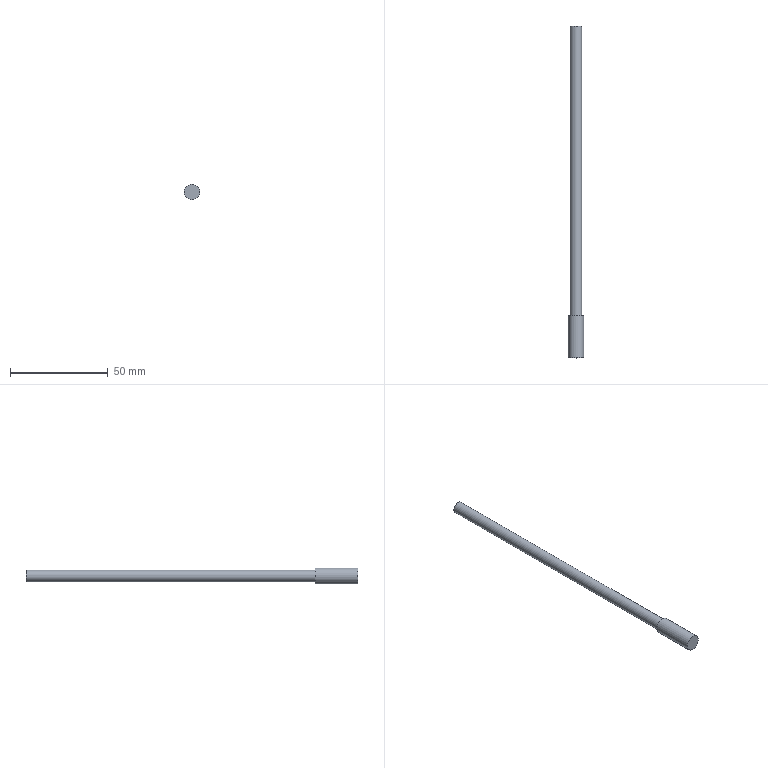Part | NX | features solid 2 | 1 solid | 5 faces | box 8 x 169.5 x 8 mm | volume 5274 mm3 | plane 3 | cylinder 2 | commonest cylinder face diameters 6 x1 8 x1
STEP:
#1=CARTESIAN_POINT('',(67.,72.5,-32.));
#2=VERTEX_POINT('',#1);
#3=CARTESIAN_POINT('',(67.,72.5,-35.));
#4=DIRECTION('',(0.,1.,0.));
#5=DIRECTION('',(0.,0.,1.));
#6=AXIS2_PLACEMENT_3D('',#3,#4,#5);
#7=CIRCLE('',#6,3.);
#8=EDGE_CURVE('',#2,#2,#7,.F.);
#9=ORIENTED_EDGE('',*,*,#8,.T.);
#10=EDGE_LOOP('',(#9));
#11=FACE_BOUND('',#10,.T.);
#12=CARTESIAN_POINT('',(67.,-75.1,-38.));
#13=VERTEX_POINT('',#12);
#14=CARTESIAN_POINT('',(67.,-75.1,-35.));
#15=DIRECTION('',(0.,-1.,0.));
#16=DIRECTION('',(0.,0.,-1.));
#17=AXIS2_PLACEMENT_3D('',#14,#15,#16);
#18=CIRCLE('',#17,3.);
#19=EDGE_CURVE('',#13,#13,#18,.F.);
#20=ORIENTED_EDGE('',*,*,#19,.T.);
#21=EDGE_LOOP('',(#20));
#22=FACE_BOUND('',#21,.T.);
#23=CARTESIAN_POINT('',(67.,-69.,-35.));
#24=DIRECTION('',(0.,1.,0.));
#25=DIRECTION('',(1.,0.,0.));
#26=AXIS2_PLACEMENT_3D('',#23,#24,#25);
#27=CYLINDRICAL_SURFACE('',#26,3.);
#28=ADVANCED_FACE('',(#11,#22),#27,.T.);
#29=ORIENTED_EDGE('',*,*,#8,.F.);
#30=EDGE_LOOP('',(#29));
#31=FACE_BOUND('',#30,.T.);
#32=CARTESIAN_POINT('',(62.5,72.5,-50.));
#33=DIRECTION('',(0.,1.,0.));
#34=DIRECTION('',(0.,0.,1.));
#35=AXIS2_PLACEMENT_3D('',#32,#33,#34);
#36=PLANE('',#35);
#37=ADVANCED_FACE('',(#31),#36,.T.);
#38=CARTESIAN_POINT('',(67.,-75.1,-39.));
#39=VERTEX_POINT('',#38);
#40=CARTESIAN_POINT('',(67.,-75.1,-35.));
#41=DIRECTION('',(0.,-1.,0.));
#42=DIRECTION('',(0.,0.,-1.));
#43=AXIS2_PLACEMENT_3D('',#40,#41,#42);
#44=CIRCLE('',#43,4.);
#45=EDGE_CURVE('',#39,#39,#44,.T.);
#46=ORIENTED_EDGE('',*,*,#45,.T.);
#47=EDGE_LOOP('',(#46));
#48=FACE_BOUND('',#47,.T.);
#49=CARTESIAN_POINT('',(67.,-97.,-39.));
#50=VERTEX_POINT('',#49);
#51=CARTESIAN_POINT('',(67.,-97.,-35.));
#52=DIRECTION('',(0.,-1.,0.));
#53=DIRECTION('',(0.,0.,-1.));
#54=AXIS2_PLACEMENT_3D('',#51,#52,#53);
#55=CIRCLE('',#54,4.);
#56=EDGE_CURVE('',#50,#50,#55,.T.);
#57=ORIENTED_EDGE('',*,*,#56,.F.);
#58=EDGE_LOOP('',(#57));
#59=FACE_BOUND('',#58,.T.);
#60=CARTESIAN_POINT('',(67.,-75.,-35.));
#61=DIRECTION('',(0.,-1.,0.));
#62=DIRECTION('',(0.,0.,-1.));
#63=AXIS2_PLACEMENT_3D('',#60,#61,#62);
#64=CYLINDRICAL_SURFACE('',#63,4.);
#65=ADVANCED_FACE('',(#48,#59),#64,.T.);
#66=ORIENTED_EDGE('',*,*,#19,.F.);
#67=EDGE_LOOP('',(#66));
#68=FACE_BOUND('',#67,.T.);
#69=ORIENTED_EDGE('',*,*,#45,.F.);
#70=EDGE_LOOP('',(#69));
#71=FACE_BOUND('',#70,.T.);
#72=CARTESIAN_POINT('',(67.,-75.1,-35.));
#73=DIRECTION('',(0.,-1.,0.));
#74=DIRECTION('',(0.,0.,-1.));
#75=AXIS2_PLACEMENT_3D('',#72,#73,#74);
#76=PLANE('',#75);
#77=ADVANCED_FACE('',(#68,#71),#76,.F.);
#78=ORIENTED_EDGE('',*,*,#56,.T.);
#79=EDGE_LOOP('',(#78));
#80=FACE_BOUND('',#79,.T.);
#81=CARTESIAN_POINT('',(62.5,-97.,-50.));
#82=DIRECTION('',(0.,-1.,0.));
#83=DIRECTION('',(0.,0.,1.));
#84=AXIS2_PLACEMENT_3D('',#81,#82,#83);
#85=PLANE('',#84);
#86=ADVANCED_FACE('',(#80),#85,.T.);
#87=CLOSED_SHELL('',(#28,#37,#65,#77,#86));
#88=MANIFOLD_SOLID_BREP('',#87);
#89=(LENGTH_UNIT()NAMED_UNIT(*)SI_UNIT(.MILLI.,.METRE.));
#90=UNCERTAINTY_MEASURE_WITH_UNIT(LENGTH_MEASURE(0.00001),#89,'','');
#91=(NAMED_UNIT(*)PLANE_ANGLE_UNIT()SI_UNIT($,.RADIAN.));
#92=(NAMED_UNIT(*)SI_UNIT($,.STERADIAN.)SOLID_ANGLE_UNIT());
#93=(GEOMETRIC_REPRESENTATION_CONTEXT(3)GLOBAL_UNCERTAINTY_ASSIGNED_CONTEXT((#90))GLOBAL_UNIT_ASSIGNED_CONTEXT((#89,#91,#92))REPRESENTATION_CONTEXT('',''));
#94=ADVANCED_BREP_SHAPE_REPRESENTATION('',(#88),#93);